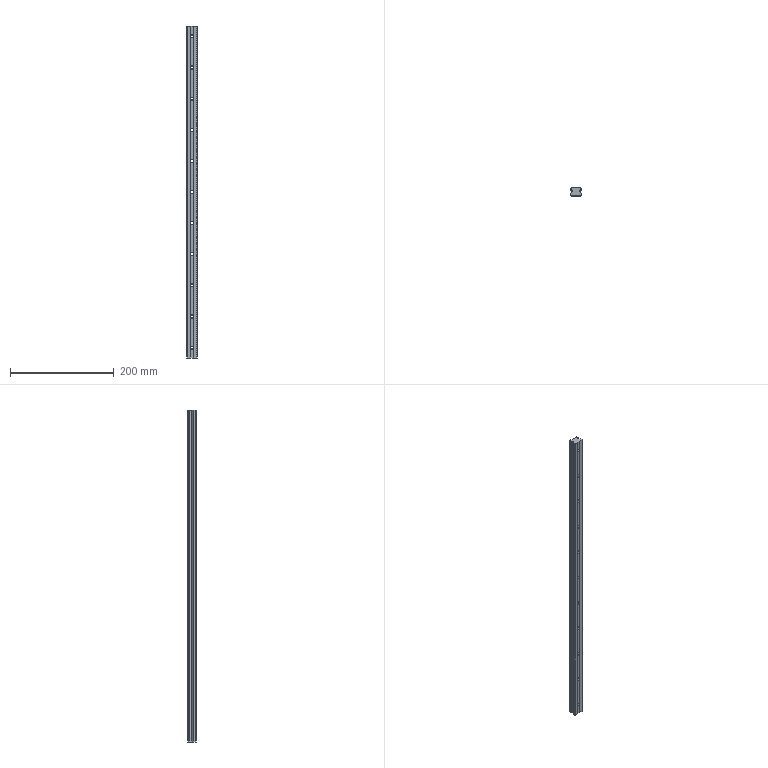Part | SolidWorks | features BaseBody 1 | 1 solid | 124 faces | box 20 x 15.5 x 640 mm | volume 170066 mm3 | plane 66 | cylinder 58 | commonest cylinder face diameters 6 x22 9.5 x22 0.6 x4 2 x4 3.5 x4 3 x2